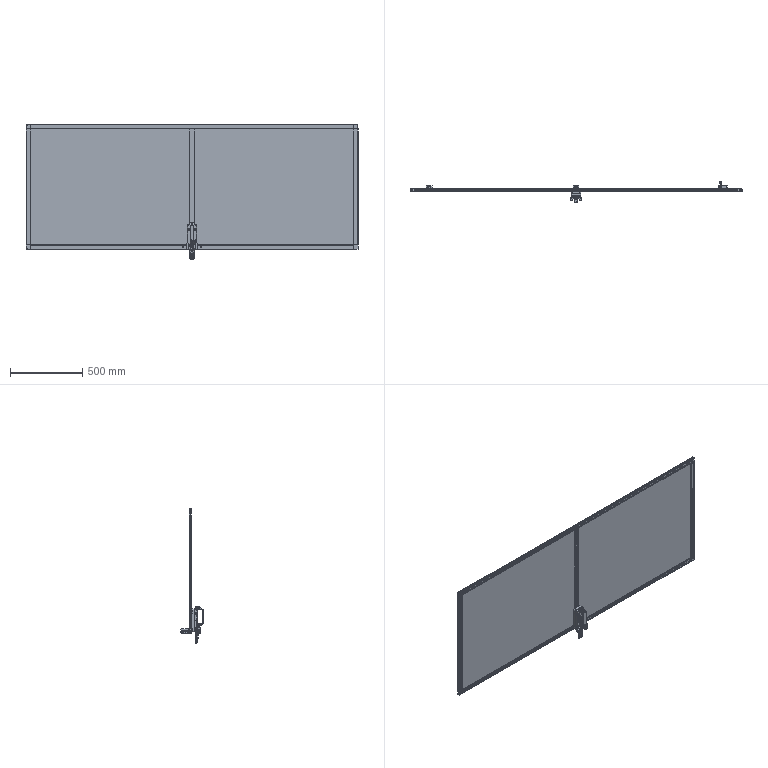Part | SolidWorks | features ReferencePattern 6, LocalLPattern 3 | 65 solids | 7113 faces | volume 11302855 mm3 | plane 4277 | cylinder 1862 | spline 557 | cone 317 | torus 68 | sphere 32 | commonest cylinder face diameters 6 x994 2 x163 1 x135 5 x117 6.5 x72 4.5 x60